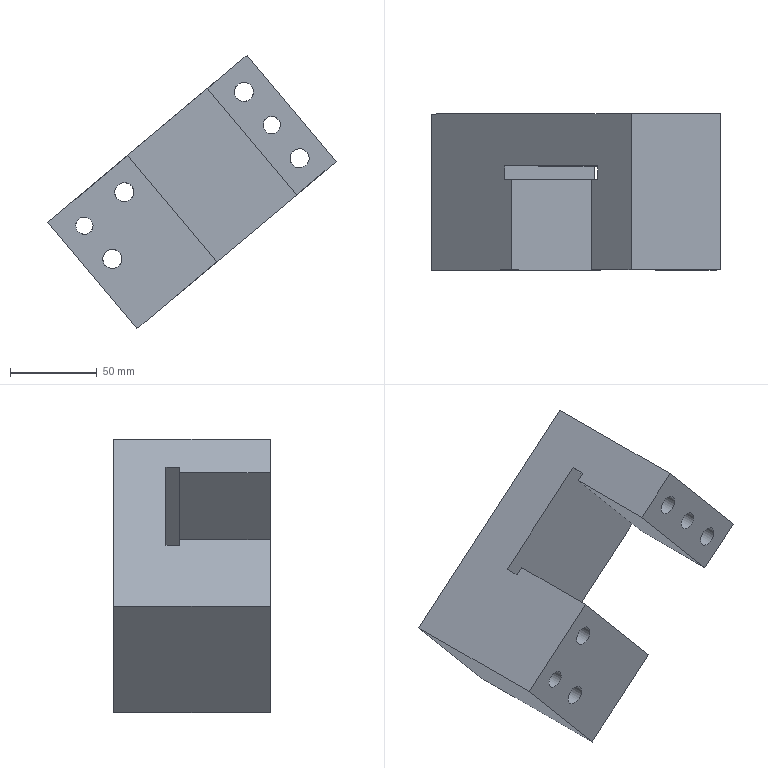Part | STEP file | solid 32 | 1 solid | 32 faces | box 166.33 x 90 x 157.702 mm | volume 730851 mm3 | plane 18 | cylinder 10 | cone 4 | commonest cylinder face diameters 11 x4 17.5 x4 10 x2